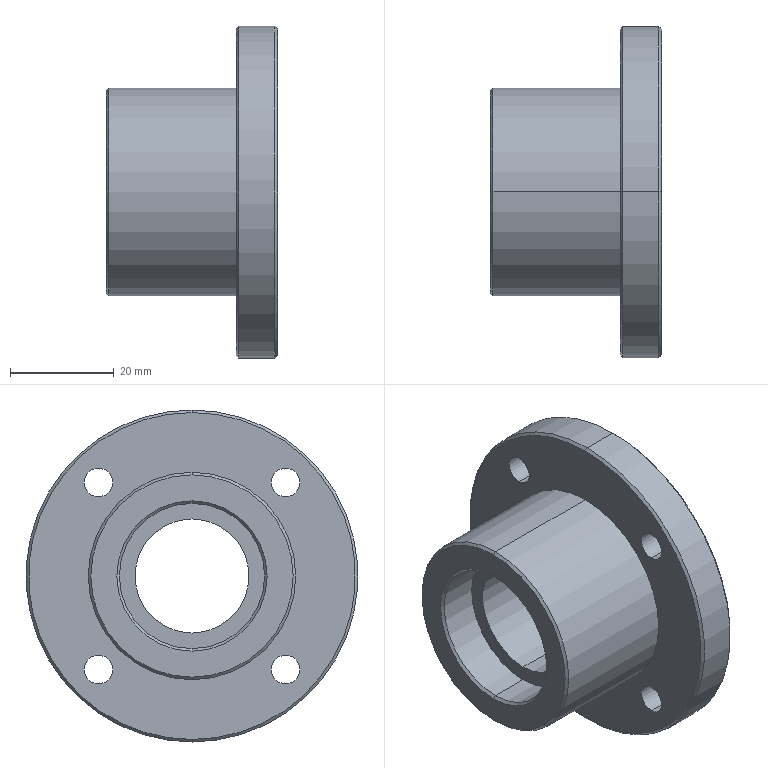Part | STEP file | PN_0033 Bearing Block_Default | 1 solid | 33 faces | box 33 x 64 x 64 mm | volume 39989 mm3 | cylinder 18 | cone 10 | plane 5 | commonest cylinder face diameters 5.5 x8 28 x4 22 x2 40 x2 64 x2